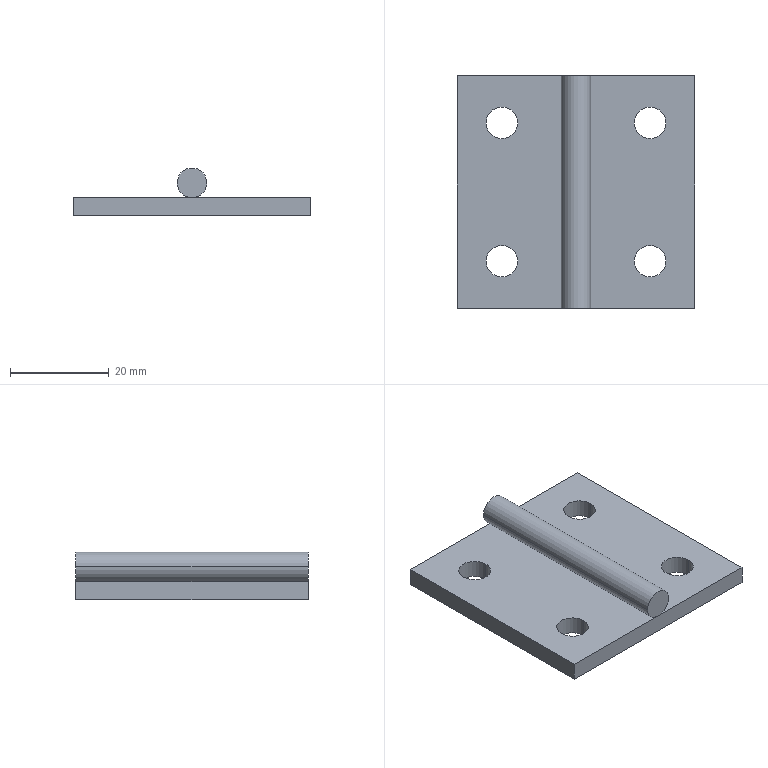Part | SolidWorks | features Extrusion 1, ICE 1 | 2 solids | 18 faces | box 48 x 47 x 9.7 mm | volume 9200 mm3 | cylinder 10 | plane 8 | commonest cylinder face diameters 6.4 x8 6 x2
STEP:
#1=CARTESIAN_POINT('',(11.8,-14.,3.7));
#2=VERTEX_POINT('',#1);
#3=CARTESIAN_POINT('',(18.2,-14.,3.7));
#4=VERTEX_POINT('',#3);
#5=CARTESIAN_POINT('',(15.,-14.,3.7));
#6=DIRECTION('',(0.,0.,1.));
#7=DIRECTION('',(1.,0.,0.));
#8=AXIS2_PLACEMENT_3D('',#5,#6,#7);
#9=CIRCLE('',#8,3.2);
#10=EDGE_CURVE('',#2,#4,#9,.T.);
#11=ORIENTED_EDGE('',*,*,#10,.T.);
#12=CARTESIAN_POINT('',(18.2,-14.,0.));
#13=VERTEX_POINT('',#12);
#14=CARTESIAN_POINT('',(18.2,-14.,3.7));
#15=DIRECTION('',(0.,0.,-1.));
#16=VECTOR('',#15,1000.);
#17=LINE('',#14,#16);
#18=EDGE_CURVE('',#4,#13,#17,.T.);
#19=ORIENTED_EDGE('',*,*,#18,.T.);
#20=CARTESIAN_POINT('',(11.8,-14.,0.));
#21=VERTEX_POINT('',#20);
#22=CARTESIAN_POINT('',(15.,-14.,0.));
#23=DIRECTION('',(0.,0.,1.));
#24=DIRECTION('',(1.,0.,0.));
#25=AXIS2_PLACEMENT_3D('',#22,#23,#24);
#26=CIRCLE('',#25,3.2);
#27=EDGE_CURVE('',#21,#13,#26,.T.);
#28=ORIENTED_EDGE('',*,*,#27,.F.);
#29=CARTESIAN_POINT('',(11.8,-14.,3.7));
#30=DIRECTION('',(0.,0.,-1.));
#31=VECTOR('',#30,1000.);
#32=LINE('',#29,#31);
#33=EDGE_CURVE('',#2,#21,#32,.T.);
#34=ORIENTED_EDGE('',*,*,#33,.F.);
#35=EDGE_LOOP('',(#11,#19,#28,#34));
#36=FACE_OUTER_BOUND('',#35,.T.);
#37=CARTESIAN_POINT('',(15.,-14.,3.7));
#38=DIRECTION('',(0.,0.,-1.));
#39=DIRECTION('',(-1.,0.,0.));
#40=AXIS2_PLACEMENT_3D('',#37,#38,#39);
#41=CYLINDRICAL_SURFACE('',#40,3.2);
#42=ADVANCED_FACE('',(#36),#41,.F.);
#43=CARTESIAN_POINT('',(11.8,14.,3.7));
#44=VERTEX_POINT('',#43);
#45=CARTESIAN_POINT('',(18.2,14.,3.7));
#46=VERTEX_POINT('',#45);
#47=CARTESIAN_POINT('',(15.,14.,3.7));
#48=DIRECTION('',(0.,0.,1.));
#49=DIRECTION('',(1.,0.,0.));
#50=AXIS2_PLACEMENT_3D('',#47,#48,#49);
#51=CIRCLE('',#50,3.2);
#52=EDGE_CURVE('',#44,#46,#51,.T.);
#53=ORIENTED_EDGE('',*,*,#52,.T.);
#54=CARTESIAN_POINT('',(18.2,14.,0.));
#55=VERTEX_POINT('',#54);
#56=CARTESIAN_POINT('',(18.2,14.,3.7));
#57=DIRECTION('',(0.,0.,-1.));
#58=VECTOR('',#57,1000.);
#59=LINE('',#56,#58);
#60=EDGE_CURVE('',#46,#55,#59,.T.);
#61=ORIENTED_EDGE('',*,*,#60,.T.);
#62=CARTESIAN_POINT('',(11.8,14.,0.));
#63=VERTEX_POINT('',#62);
#64=CARTESIAN_POINT('',(15.,14.,0.));
#65=DIRECTION('',(0.,0.,1.));
#66=DIRECTION('',(1.,0.,0.));
#67=AXIS2_PLACEMENT_3D('',#64,#65,#66);
#68=CIRCLE('',#67,3.2);
#69=EDGE_CURVE('',#63,#55,#68,.T.);
#70=ORIENTED_EDGE('',*,*,#69,.F.);
#71=CARTESIAN_POINT('',(11.8,14.,3.7));
#72=DIRECTION('',(0.,0.,-1.));
#73=VECTOR('',#72,1000.);
#74=LINE('',#71,#73);
#75=EDGE_CURVE('',#44,#63,#74,.T.);
#76=ORIENTED_EDGE('',*,*,#75,.F.);
#77=EDGE_LOOP('',(#53,#61,#70,#76));
#78=FACE_OUTER_BOUND('',#77,.T.);
#79=CARTESIAN_POINT('',(15.,14.,3.7));
#80=DIRECTION('',(0.,0.,-1.));
#81=DIRECTION('',(-1.,0.,0.));
#82=AXIS2_PLACEMENT_3D('',#79,#80,#81);
#83=CYLINDRICAL_SURFACE('',#82,3.2);
#84=ADVANCED_FACE('',(#78),#83,.F.);
#85=CARTESIAN_POINT('',(-18.2,-14.,3.7));
#86=VERTEX_POINT('',#85);
#87=CARTESIAN_POINT('',(-11.8,-14.,3.7));
#88=VERTEX_POINT('',#87);
#89=CARTESIAN_POINT('',(-15.,-14.,3.7));
#90=DIRECTION('',(0.,0.,1.));
#91=DIRECTION('',(1.,0.,0.));
#92=AXIS2_PLACEMENT_3D('',#89,#90,#91);
#93=CIRCLE('',#92,3.2);
#94=EDGE_CURVE('',#86,#88,#93,.T.);
#95=ORIENTED_EDGE('',*,*,#94,.T.);
#96=CARTESIAN_POINT('',(-11.8,-14.,0.));
#97=VERTEX_POINT('',#96);
#98=CARTESIAN_POINT('',(-11.8,-14.,3.7));
#99=DIRECTION('',(0.,0.,-1.));
#100=VECTOR('',#99,1000.);
#101=LINE('',#98,#100);
#102=EDGE_CURVE('',#88,#97,#101,.T.);
#103=ORIENTED_EDGE('',*,*,#102,.T.);
#104=CARTESIAN_POINT('',(-18.2,-14.,0.));
#105=VERTEX_POINT('',#104);
#106=CARTESIAN_POINT('',(-15.,-14.,0.));
#107=DIRECTION('',(0.,0.,1.));
#108=DIRECTION('',(1.,0.,0.));
#109=AXIS2_PLACEMENT_3D('',#106,#107,#108);
#110=CIRCLE('',#109,3.2);
#111=EDGE_CURVE('',#105,#97,#110,.T.);
#112=ORIENTED_EDGE('',*,*,#111,.F.);
#113=CARTESIAN_POINT('',(-18.2,-14.,3.7));
#114=DIRECTION('',(0.,0.,-1.));
#115=VECTOR('',#114,1000.);
#116=LINE('',#113,#115);
#117=EDGE_CURVE('',#86,#105,#116,.T.);
#118=ORIENTED_EDGE('',*,*,#117,.F.);
#119=EDGE_LOOP('',(#95,#103,#112,#118));
#120=FACE_OUTER_BOUND('',#119,.T.);
#121=CARTESIAN_POINT('',(-15.,-14.,3.7));
#122=DIRECTION('',(0.,0.,-1.));
#123=DIRECTION('',(-1.,0.,0.));
#124=AXIS2_PLACEMENT_3D('',#121,#122,#123);
#125=CYLINDRICAL_SURFACE('',#124,3.2);
#126=ADVANCED_FACE('',(#120),#125,.F.);
#127=CARTESIAN_POINT('',(-18.2,14.,3.7));
#128=VERTEX_POINT('',#127);
#129=CARTESIAN_POINT('',(-11.8,14.,3.7));
#130=VERTEX_POINT('',#129);
#131=CARTESIAN_POINT('',(-15.,14.,3.7));
#132=DIRECTION('',(0.,0.,1.));
#133=DIRECTION('',(1.,0.,0.));
#134=AXIS2_PLACEMENT_3D('',#131,#132,#133);
#135=CIRCLE('',#134,3.2);
#136=EDGE_CURVE('',#128,#130,#135,.T.);
#137=ORIENTED_EDGE('',*,*,#136,.T.);
#138=CARTESIAN_POINT('',(-11.8,14.,0.));
#139=VERTEX_POINT('',#138);
#140=CARTESIAN_POINT('',(-11.8,14.,3.7));
#141=DIRECTION('',(0.,0.,-1.));
#142=VECTOR('',#141,1000.);
#143=LINE('',#140,#142);
#144=EDGE_CURVE('',#130,#139,#143,.T.);
#145=ORIENTED_EDGE('',*,*,#144,.T.);
#146=CARTESIAN_POINT('',(-18.2,14.,0.));
#147=VERTEX_POINT('',#146);
#148=CARTESIAN_POINT('',(-15.,14.,0.));
#149=DIRECTION('',(0.,0.,1.));
#150=DIRECTION('',(1.,0.,0.));
#151=AXIS2_PLACEMENT_3D('',#148,#149,#150);
#152=CIRCLE('',#151,3.2);
#153=EDGE_CURVE('',#147,#139,#152,.T.);
#154=ORIENTED_EDGE('',*,*,#153,.F.);
#155=CARTESIAN_POINT('',(-18.2,14.,3.7));
#156=DIRECTION('',(0.,0.,-1.));
#157=VECTOR('',#156,1000.);
#158=LINE('',#155,#157);
#159=EDGE_CURVE('',#128,#147,#158,.T.);
#160=ORIENTED_EDGE('',*,*,#159,.F.);
#161=EDGE_LOOP('',(#137,#145,#154,#160));
#162=FACE_OUTER_BOUND('',#161,.T.);
#163=CARTESIAN_POINT('',(-15.,14.,3.7));
#164=DIRECTION('',(0.,0.,-1.));
#165=DIRECTION('',(-1.,0.,0.));
#166=AXIS2_PLACEMENT_3D('',#163,#164,#165);
#167=CYLINDRICAL_SURFACE('',#166,3.2);
#168=ADVANCED_FACE('',(#162),#167,.F.);
#169=CARTESIAN_POINT('',(-24.,-23.5,3.7));
#170=VERTEX_POINT('',#169);
#171=CARTESIAN_POINT('',(24.,-23.5,3.7));
#172=VERTEX_POINT('',#171);
#173=CARTESIAN_POINT('',(-24.,-23.5,3.7));
#174=DIRECTION('',(1.,0.,0.));
#175=VECTOR('',#174,1000.);
#176=LINE('',#173,#175);
#177=EDGE_CURVE('',#170,#172,#176,.T.);
#178=ORIENTED_EDGE('',*,*,#177,.T.);
#179=CARTESIAN_POINT('',(24.,23.5,3.7));
#180=VERTEX_POINT('',#179);
#181=CARTESIAN_POINT('',(24.,23.5,3.7));
#182=DIRECTION('',(0.,1.,0.));
#183=VECTOR('',#182,1000.);
#184=LINE('',#181,#183);
#185=EDGE_CURVE('',#172,#180,#184,.T.);
#186=ORIENTED_EDGE('',*,*,#185,.T.);
#187=CARTESIAN_POINT('',(-24.,23.5,3.7));
#188=VERTEX_POINT('',#187);
#189=CARTESIAN_POINT('',(-24.,23.5,3.7));
#190=DIRECTION('',(-1.,0.,0.));
#191=VECTOR('',#190,1000.);
#192=LINE('',#189,#191);
#193=EDGE_CURVE('',#180,#188,#192,.T.);
#194=ORIENTED_EDGE('',*,*,#193,.T.);
#195=CARTESIAN_POINT('',(-24.,23.5,3.7));
#196=DIRECTION('',(0.,-1.,0.));
#197=VECTOR('',#196,1000.);
#198=LINE('',#195,#197);
#199=EDGE_CURVE('',#188,#170,#198,.T.);
#200=ORIENTED_EDGE('',*,*,#199,.T.);
#201=EDGE_LOOP('',(#178,#186,#194,#200));
#202=FACE_OUTER_BOUND('',#201,.T.);
#203=ORIENTED_EDGE('',*,*,#136,.F.);
#204=CARTESIAN_POINT('',(-15.,14.,3.7));
#205=DIRECTION('',(0.,0.,1.));
#206=DIRECTION('',(1.,0.,0.));
#207=AXIS2_PLACEMENT_3D('',#204,#205,#206);
#208=CIRCLE('',#207,3.2);
#209=EDGE_CURVE('',#130,#128,#208,.T.);
#210=ORIENTED_EDGE('',*,*,#209,.F.);
#211=EDGE_LOOP('',(#203,#210));
#212=FACE_BOUND('',#211,.T.);
#213=ORIENTED_EDGE('',*,*,#94,.F.);
#214=CARTESIAN_POINT('',(-15.,-14.,3.7));
#215=DIRECTION('',(0.,0.,1.));
#216=DIRECTION('',(1.,0.,0.));
#217=AXIS2_PLACEMENT_3D('',#214,#215,#216);
#218=CIRCLE('',#217,3.2);
#219=EDGE_CURVE('',#88,#86,#218,.T.);
#220=ORIENTED_EDGE('',*,*,#219,.F.);
#221=EDGE_LOOP('',(#213,#220));
#222=FACE_BOUND('',#221,.T.);
#223=ORIENTED_EDGE('',*,*,#10,.F.);
#224=CARTESIAN_POINT('',(15.,-14.,3.7));
#225=DIRECTION('',(0.,0.,1.));
#226=DIRECTION('',(1.,0.,0.));
#227=AXIS2_PLACEMENT_3D('',#224,#225,#226);
#228=CIRCLE('',#227,3.2);
#229=EDGE_CURVE('',#4,#2,#228,.T.);
#230=ORIENTED_EDGE('',*,*,#229,.F.);
#231=EDGE_LOOP('',(#223,#230));
#232=FACE_BOUND('',#231,.T.);
#233=ORIENTED_EDGE('',*,*,#52,.F.);
#234=CARTESIAN_POINT('',(15.,14.,3.7));
#235=DIRECTION('',(0.,0.,1.));
#236=DIRECTION('',(1.,0.,0.));
#237=AXIS2_PLACEMENT_3D('',#234,#235,#236);
#238=CIRCLE('',#237,3.2);
#239=EDGE_CURVE('',#46,#44,#238,.T.);
#240=ORIENTED_EDGE('',*,*,#239,.F.);
#241=EDGE_LOOP('',(#233,#240));
#242=FACE_BOUND('',#241,.T.);
#243=CARTESIAN_POINT('',(0.,0.,3.7));
#244=DIRECTION('',(0.,0.,1.));
#245=DIRECTION('',(1.,0.,0.));
#246=AXIS2_PLACEMENT_3D('',#243,#244,#245);
#247=PLANE('',#246);
#248=ADVANCED_FACE('',(#202,#212,#222,#232,#242),#247,.T.);
#249=ORIENTED_EDGE('',*,*,#69,.T.);
#250=CARTESIAN_POINT('',(15.,14.,0.));
#251=DIRECTION('',(0.,0.,1.));
#252=DIRECTION('',(1.,0.,0.));
#253=AXIS2_PLACEMENT_3D('',#250,#251,#252);
#254=CIRCLE('',#253,3.2);
#255=EDGE_CURVE('',#55,#63,#254,.T.);
#256=ORIENTED_EDGE('',*,*,#255,.T.);
#257=EDGE_LOOP('',(#249,#256));
#258=FACE_BOUND('',#257,.T.);
#259=ORIENTED_EDGE('',*,*,#153,.T.);
#260=CARTESIAN_POINT('',(-15.,14.,0.));
#261=DIRECTION('',(0.,0.,1.));
#262=DIRECTION('',(1.,0.,0.));
#263=AXIS2_PLACEMENT_3D('',#260,#261,#262);
#264=CIRCLE('',#263,3.2);
#265=EDGE_CURVE('',#139,#147,#264,.T.);
#266=ORIENTED_EDGE('',*,*,#265,.T.);
#267=EDGE_LOOP('',(#259,#266));
#268=FACE_BOUND('',#267,.T.);
#269=CARTESIAN_POINT('',(24.,-23.5,0.));
#270=VERTEX_POINT('',#269);
#271=CARTESIAN_POINT('',(24.,23.5,0.));
#272=VERTEX_POINT('',#271);
#273=CARTESIAN_POINT('',(24.,23.5,0.));
#274=DIRECTION('',(0.,1.,0.));
#275=VECTOR('',#274,1000.);
#276=LINE('',#273,#275);
#277=EDGE_CURVE('',#270,#272,#276,.T.);
#278=ORIENTED_EDGE('',*,*,#277,.F.);
#279=CARTESIAN_POINT('',(-24.,-23.5,0.));
#280=VERTEX_POINT('',#279);
#281=CARTESIAN_POINT('',(-24.,-23.5,0.));
#282=DIRECTION('',(1.,0.,0.));
#283=VECTOR('',#282,1000.);
#284=LINE('',#281,#283);
#285=EDGE_CURVE('',#280,#270,#284,.T.);
#286=ORIENTED_EDGE('',*,*,#285,.F.);
#287=CARTESIAN_POINT('',(-24.,23.5,0.));
#288=VERTEX_POINT('',#287);
#289=CARTESIAN_POINT('',(-24.,23.5,0.));
#290=DIRECTION('',(0.,-1.,0.));
#291=VECTOR('',#290,1000.);
#292=LINE('',#289,#291);
#293=EDGE_CURVE('',#288,#280,#292,.T.);
#294=ORIENTED_EDGE('',*,*,#293,.F.);
#295=CARTESIAN_POINT('',(-24.,23.5,0.));
#296=DIRECTION('',(-1.,0.,0.));
#297=VECTOR('',#296,1000.);
#298=LINE('',#295,#297);
#299=EDGE_CURVE('',#272,#288,#298,.T.);
#300=ORIENTED_EDGE('',*,*,#299,.F.);
#301=EDGE_LOOP('',(#278,#286,#294,#300));
#302=FACE_OUTER_BOUND('',#301,.T.);
#303=ORIENTED_EDGE('',*,*,#111,.T.);
#304=CARTESIAN_POINT('',(-15.,-14.,0.));
#305=DIRECTION('',(0.,0.,1.));
#306=DIRECTION('',(1.,0.,0.));
#307=AXIS2_PLACEMENT_3D('',#304,#305,#306);
#308=CIRCLE('',#307,3.2);
#309=EDGE_CURVE('',#97,#105,#308,.T.);
#310=ORIENTED_EDGE('',*,*,#309,.T.);
#311=EDGE_LOOP('',(#303,#310));
#312=FACE_BOUND('',#311,.T.);
#313=ORIENTED_EDGE('',*,*,#27,.T.);
#314=CARTESIAN_POINT('',(15.,-14.,0.));
#315=DIRECTION('',(0.,0.,1.));
#316=DIRECTION('',(1.,0.,0.));
#317=AXIS2_PLACEMENT_3D('',#314,#315,#316);
#318=CIRCLE('',#317,3.2);
#319=EDGE_CURVE('',#13,#21,#318,.T.);
#320=ORIENTED_EDGE('',*,*,#319,.T.);
#321=EDGE_LOOP('',(#313,#320));
#322=FACE_BOUND('',#321,.T.);
#323=CARTESIAN_POINT('',(0.,0.,0.));
#324=DIRECTION('',(0.,0.,1.));
#325=DIRECTION('',(1.,0.,0.));
#326=AXIS2_PLACEMENT_3D('',#323,#324,#325);
#327=PLANE('',#326);
#328=ADVANCED_FACE('',(#258,#268,#302,#312,#322),#327,.F.);
#329=ORIENTED_EDGE('',*,*,#277,.T.);
#330=CARTESIAN_POINT('',(24.,23.5,3.7));
#331=DIRECTION('',(0.,0.,-1.));
#332=VECTOR('',#331,1000.);
#333=LINE('',#330,#332);
#334=EDGE_CURVE('',#180,#272,#333,.T.);
#335=ORIENTED_EDGE('',*,*,#334,.F.);
#336=ORIENTED_EDGE('',*,*,#185,.F.);
#337=CARTESIAN_POINT('',(24.,-23.5,3.7));
#338=DIRECTION('',(0.,0.,-1.));
#339=VECTOR('',#338,1000.);
#340=LINE('',#337,#339);
#341=EDGE_CURVE('',#172,#270,#340,.T.);
#342=ORIENTED_EDGE('',*,*,#341,.T.);
#343=EDGE_LOOP('',(#329,#335,#336,#342));
#344=FACE_OUTER_BOUND('',#343,.T.);
#345=CARTESIAN_POINT('',(24.,23.5,3.7));
#346=DIRECTION('',(-1.,0.,0.));
#347=DIRECTION('',(0.,-1.,0.));
#348=AXIS2_PLACEMENT_3D('',#345,#346,#347);
#349=PLANE('',#348);
#350=ADVANCED_FACE('',(#344),#349,.F.);
#351=ORIENTED_EDGE('',*,*,#299,.T.);
#352=CARTESIAN_POINT('',(-24.,23.5,3.7));
#353=DIRECTION('',(0.,0.,-1.));
#354=VECTOR('',#353,1000.);
#355=LINE('',#352,#354);
#356=EDGE_CURVE('',#188,#288,#355,.T.);
#357=ORIENTED_EDGE('',*,*,#356,.F.);
#358=ORIENTED_EDGE('',*,*,#193,.F.);
#359=ORIENTED_EDGE('',*,*,#334,.T.);
#360=EDGE_LOOP('',(#351,#357,#358,#359));
#361=FACE_OUTER_BOUND('',#360,.T.);
#362=CARTESIAN_POINT('',(-24.,23.5,3.7));
#363=DIRECTION('',(0.,-1.,0.));
#364=DIRECTION('',(0.,0.,-1.));
#365=AXIS2_PLACEMENT_3D('',#362,#363,#364);
#366=PLANE('',#365);
#367=ADVANCED_FACE('',(#361),#366,.F.);
#368=ORIENTED_EDGE('',*,*,#293,.T.);
#369=CARTESIAN_POINT('',(-24.,-23.5,3.7));
#370=DIRECTION('',(0.,0.,-1.));
#371=VECTOR('',#370,1000.);
#372=LINE('',#369,#371);
#373=EDGE_CURVE('',#170,#280,#372,.T.);
#374=ORIENTED_EDGE('',*,*,#373,.F.);
#375=ORIENTED_EDGE('',*,*,#199,.F.);
#376=ORIENTED_EDGE('',*,*,#356,.T.);
#377=EDGE_LOOP('',(#368,#374,#375,#376));
#378=FACE_OUTER_BOUND('',#377,.T.);
#379=CARTESIAN_POINT('',(-24.,23.5,3.7));
#380=DIRECTION('',(1.,0.,0.));
#381=DIRECTION('',(0.,1.,0.));
#382=AXIS2_PLACEMENT_3D('',#379,#380,#381);
#383=PLANE('',#382);
#384=ADVANCED_FACE('',(#378),#383,.F.);
#385=ORIENTED_EDGE('',*,*,#285,.T.);
#386=ORIENTED_EDGE('',*,*,#341,.F.);
#387=ORIENTED_EDGE('',*,*,#177,.F.);
#388=ORIENTED_EDGE('',*,*,#373,.T.);
#389=EDGE_LOOP('',(#385,#386,#387,#388));
#390=FACE_OUTER_BOUND('',#389,.T.);
#391=CARTESIAN_POINT('',(-24.,-23.5,3.7));
#392=DIRECTION('',(0.,1.,0.));
#393=DIRECTION('',(-1.,0.,0.));
#394=AXIS2_PLACEMENT_3D('',#391,#392,#393);
#395=PLANE('',#394);
#396=ADVANCED_FACE('',(#390),#395,.F.);
#397=ORIENTED_EDGE('',*,*,#144,.F.);
#398=ORIENTED_EDGE('',*,*,#209,.T.);
#399=ORIENTED_EDGE('',*,*,#159,.T.);
#400=ORIENTED_EDGE('',*,*,#265,.F.);
#401=EDGE_LOOP('',(#397,#398,#399,#400));
#402=FACE_OUTER_BOUND('',#401,.T.);
#403=CARTESIAN_POINT('',(-15.,14.,3.7));
#404=DIRECTION('',(0.,0.,-1.));
#405=DIRECTION('',(-1.,0.,0.));
#406=AXIS2_PLACEMENT_3D('',#403,#404,#405);
#407=CYLINDRICAL_SURFACE('',#406,3.2);
#408=ADVANCED_FACE('',(#402),#407,.F.);
#409=ORIENTED_EDGE('',*,*,#102,.F.);
#410=ORIENTED_EDGE('',*,*,#219,.T.);
#411=ORIENTED_EDGE('',*,*,#117,.T.);
#412=ORIENTED_EDGE('',*,*,#309,.F.);
#413=EDGE_LOOP('',(#409,#410,#411,#412));
#414=FACE_OUTER_BOUND('',#413,.T.);
#415=CARTESIAN_POINT('',(-15.,-14.,3.7));
#416=DIRECTION('',(0.,0.,-1.));
#417=DIRECTION('',(-1.,0.,0.));
#418=AXIS2_PLACEMENT_3D('',#415,#416,#417);
#419=CYLINDRICAL_SURFACE('',#418,3.2);
#420=ADVANCED_FACE('',(#414),#419,.F.);
#421=ORIENTED_EDGE('',*,*,#60,.F.);
#422=ORIENTED_EDGE('',*,*,#239,.T.);
#423=ORIENTED_EDGE('',*,*,#75,.T.);
#424=ORIENTED_EDGE('',*,*,#255,.F.);
#425=EDGE_LOOP('',(#421,#422,#423,#424));
#426=FACE_OUTER_BOUND('',#425,.T.);
#427=CARTESIAN_POINT('',(15.,14.,3.7));
#428=DIRECTION('',(0.,0.,-1.));
#429=DIRECTION('',(-1.,0.,0.));
#430=AXIS2_PLACEMENT_3D('',#427,#428,#429);
#431=CYLINDRICAL_SURFACE('',#430,3.2);
#432=ADVANCED_FACE('',(#426),#431,.F.);
#433=ORIENTED_EDGE('',*,*,#18,.F.);
#434=ORIENTED_EDGE('',*,*,#229,.T.);
#435=ORIENTED_EDGE('',*,*,#33,.T.);
#436=ORIENTED_EDGE('',*,*,#319,.F.);
#437=EDGE_LOOP('',(#433,#434,#435,#436));
#438=FACE_OUTER_BOUND('',#437,.T.);
#439=CARTESIAN_POINT('',(15.,-14.,3.7));
#440=DIRECTION('',(0.,0.,-1.));
#441=DIRECTION('',(-1.,0.,0.));
#442=AXIS2_PLACEMENT_3D('',#439,#440,#441);
#443=CYLINDRICAL_SURFACE('',#442,3.2);
#444=ADVANCED_FACE('',(#438),#443,.F.);
#445=CLOSED_SHELL('',(#42,#84,#126,#168,#248,#328,#350,#367,#384,#396,#408,#420,#432,#444));
#446=MANIFOLD_SOLID_BREP('',#445);
#447=CARTESIAN_POINT('',(-3.,23.5,6.7));
#448=VERTEX_POINT('',#447);
#449=CARTESIAN_POINT('',(3.,23.5,6.7));
#450=VERTEX_POINT('',#449);
#451=CARTESIAN_POINT('',(0.,23.5,6.7));
#452=DIRECTION('',(0.,1.,0.));
#453=DIRECTION('',(0.,0.,-1.));
#454=AXIS2_PLACEMENT_3D('',#451,#452,#453);
#455=CIRCLE('',#454,3.);
#456=EDGE_CURVE('',#448,#450,#455,.T.);
#457=ORIENTED_EDGE('',*,*,#456,.F.);
#458=CARTESIAN_POINT('',(-3.,-23.5,6.7));
#459=VERTEX_POINT('',#458);
#460=CARTESIAN_POINT('',(-3.,31.985,6.7));
#461=DIRECTION('',(0.,-1.,0.));
#462=VECTOR('',#461,1000.);
#463=LINE('',#460,#462);
#464=EDGE_CURVE('',#448,#459,#463,.T.);
#465=ORIENTED_EDGE('',*,*,#464,.T.);
#466=CARTESIAN_POINT('',(3.,-23.5,6.7));
#467=VERTEX_POINT('',#466);
#468=CARTESIAN_POINT('',(0.,-23.5,6.7));
#469=DIRECTION('',(0.,-1.,0.));
#470=DIRECTION('',(1.,0.,0.));
#471=AXIS2_PLACEMENT_3D('',#468,#469,#470);
#472=CIRCLE('',#471,3.);
#473=EDGE_CURVE('',#467,#459,#472,.T.);
#474=ORIENTED_EDGE('',*,*,#473,.F.);
#475=CARTESIAN_POINT('',(3.,31.985,6.7));
#476=DIRECTION('',(0.,-1.,0.));
#477=VECTOR('',#476,1000.);
#478=LINE('',#475,#477);
#479=EDGE_CURVE('',#450,#467,#478,.T.);
#480=ORIENTED_EDGE('',*,*,#479,.F.);
#481=EDGE_LOOP('',(#457,#465,#474,#480));
#482=FACE_OUTER_BOUND('',#481,.T.);
#483=CARTESIAN_POINT('',(0.,31.985,6.7));
#484=DIRECTION('',(0.,-1.,0.));
#485=DIRECTION('',(1.,0.,0.));
#486=AXIS2_PLACEMENT_3D('',#483,#484,#485);
#487=CYLINDRICAL_SURFACE('',#486,3.);
#488=ADVANCED_FACE('',(#482),#487,.T.);
#489=ORIENTED_EDGE('',*,*,#464,.F.);
#490=CARTESIAN_POINT('',(0.,23.5,6.7));
#491=DIRECTION('',(0.,1.,0.));
#492=DIRECTION('',(0.,0.,-1.));
#493=AXIS2_PLACEMENT_3D('',#490,#491,#492);
#494=CIRCLE('',#493,3.);
#495=EDGE_CURVE('',#450,#448,#494,.T.);
#496=ORIENTED_EDGE('',*,*,#495,.F.);
#497=ORIENTED_EDGE('',*,*,#479,.T.);
#498=CARTESIAN_POINT('',(0.,-23.5,6.7));
#499=DIRECTION('',(0.,-1.,0.));
#500=DIRECTION('',(1.,0.,0.));
#501=AXIS2_PLACEMENT_3D('',#498,#499,#500);
#502=CIRCLE('',#501,3.);
#503=EDGE_CURVE('',#459,#467,#502,.T.);
#504=ORIENTED_EDGE('',*,*,#503,.F.);
#505=EDGE_LOOP('',(#489,#496,#497,#504));
#506=FACE_OUTER_BOUND('',#505,.T.);
#507=CARTESIAN_POINT('',(0.,31.985,6.7));
#508=DIRECTION('',(0.,-1.,0.));
#509=DIRECTION('',(1.,0.,0.));
#510=AXIS2_PLACEMENT_3D('',#507,#508,#509);
#511=CYLINDRICAL_SURFACE('',#510,3.);
#512=ADVANCED_FACE('',(#506),#511,.T.);
#513=ORIENTED_EDGE('',*,*,#473,.T.);
#514=ORIENTED_EDGE('',*,*,#503,.T.);
#515=EDGE_LOOP('',(#513,#514));
#516=FACE_OUTER_BOUND('',#515,.T.);
#517=CARTESIAN_POINT('',(0.,-23.5,6.7));
#518=DIRECTION('',(0.,-1.,0.));
#519=DIRECTION('',(1.,0.,0.));
#520=AXIS2_PLACEMENT_3D('',#517,#518,#519);
#521=PLANE('',#520);
#522=ADVANCED_FACE('',(#516),#521,.T.);
#523=ORIENTED_EDGE('',*,*,#495,.T.);
#524=ORIENTED_EDGE('',*,*,#456,.T.);
#525=EDGE_LOOP('',(#523,#524));
#526=FACE_OUTER_BOUND('',#525,.T.);
#527=CARTESIAN_POINT('',(-24.,23.5,3.7));
#528=DIRECTION('',(0.,-1.,0.));
#529=DIRECTION('',(0.,0.,-1.));
#530=AXIS2_PLACEMENT_3D('',#527,#528,#529);
#531=PLANE('',#530);
#532=ADVANCED_FACE('',(#526),#531,.F.);
#533=CLOSED_SHELL('',(#488,#512,#522,#532));
#534=MANIFOLD_SOLID_BREP('',#533);
#535=CARTESIAN_POINT('',(0.,0.,0.));
#536=DIRECTION('',(0.,0.,1.));
#537=DIRECTION('',(1.,0.,0.));
#538=AXIS2_PLACEMENT_3D('',#535,#536,#537);
#539=(LENGTH_UNIT()NAMED_UNIT(*)SI_UNIT(.MILLI.,.METRE.));
#540=UNCERTAINTY_MEASURE_WITH_UNIT(LENGTH_MEASURE(0.00001),#539,'','');
#541=(NAMED_UNIT(*)PLANE_ANGLE_UNIT()SI_UNIT($,.RADIAN.));
#542=(NAMED_UNIT(*)SI_UNIT($,.STERADIAN.)SOLID_ANGLE_UNIT());
#543=(GEOMETRIC_REPRESENTATION_CONTEXT(3)GLOBAL_UNCERTAINTY_ASSIGNED_CONTEXT((#540))GLOBAL_UNIT_ASSIGNED_CONTEXT((#539,#541,#542))REPRESENTATION_CONTEXT('',''));
#544=ADVANCED_BREP_SHAPE_REPRESENTATION('',(#446,#534,#538),#543);